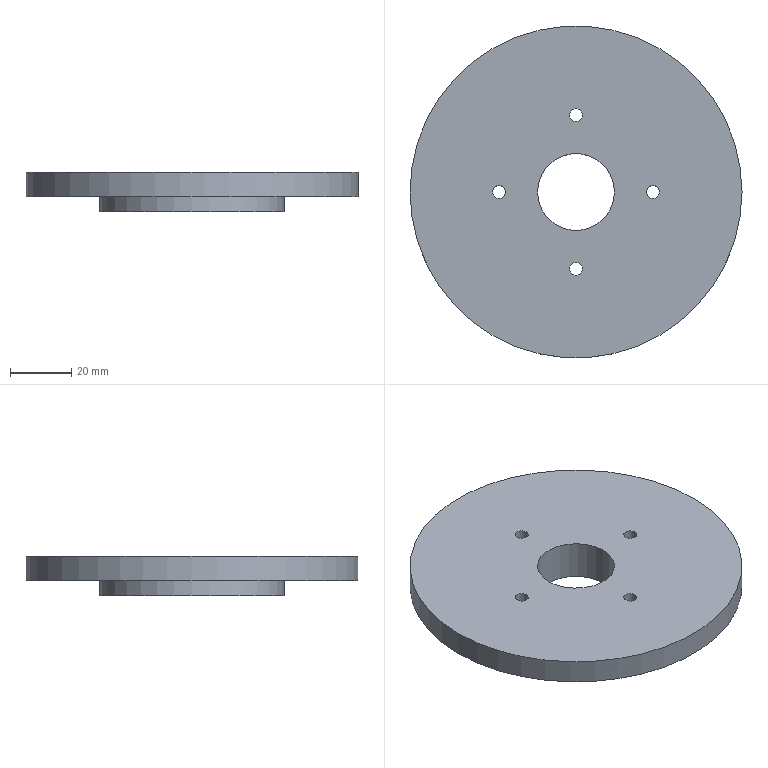NC program | NX | posted with a generic post | part box 108 x 108 x 13 mm
Whole program:
N10 G17 G21 G94 G90
(DRILLING , TOOL : ZXZ)
N12 T01 M6
N14 G54
N16 G17 G0 G90 X-25. Y0. S3000 M3
N18 G43 Z30. H1
N20 G94 G81 G98 Z-1. F200. R3.
N22 X0. Y-25.
N24 X25. Y0.
N26 X0. Y25.
N28 G80
N30 G0 X0. Y25. Z30.
N32 M5
(DRILLING_COPY , TOOL : 4.2ZT)
N34 T02 M6
N36 G54
N38 G17 G0 G90 X-25. Y0. S2000 M3
N40 G43 Z30. H2
N42 G94 G83 G98 Z-15.762 F110. Q2. R3.
N44 X0. Y-25.
N46 X25. Y0.
N48 X0. Y25.
N50 G80
N52 G0 X0. Y25. Z30.
N54 M5
(ZLEVEL_PROFILE_1_COPY_1 , TOOL : D6A45)
N56 T07 M6
N58 G54
N60 G17 G0 G90 X-25.021 Y0.012 S7500 M3
N62 G43 Z30. H7
N64 Z0.
N66 G94 G1 Z-1. F1000.
N68 X-25.924 Y0.52
N70 G3 X-26.224 Y0. R0.6
N72 X-25. Y-1.224 R1.224
N74 X-26.224 Y0. R-1.224
N76 X-25.924 Y-0.52 R0.6
N78 G1 X-25.021 Y-0.012
N80 Z0.
N82 G0 Z30.
N84 X0.012 Y25.021
N86 Z0.
N88 G1 Z-1.
N90 X0.52 Y25.924
N92 G3 X0. Y26.224 R0.6
N94 X-1.224 Y25. R1.224
N96 X0. Y26.224 R-1.224
N98 X-0.52 Y25.924 R0.6
N100 G1 X-0.012 Y25.021
N102 Z0.
N104 G0 Z30.
N106 Y-25.021
N108 Z0.
N110 G1 Z-1.
N112 X-0.52 Y-25.924
N114 G3 X0. Y-26.224 R0.6
N116 X1.224 Y-25. R1.224
N118 X0. Y-26.224 R-1.224
N120 X0.52 Y-25.924 R0.6
N122 G1 X0.012 Y-25.021
N124 Z0.
N126 G0 Z30.
N128 X25.021 Y-0.012
N130 Z0.
N132 G1 Z-1.
N134 X25.924 Y-0.52
N136 G3 X26.224 Y0. R0.6
N138 X25. Y1.224 R1.224
N140 X26.224 Y0. R-1.224
N142 X25.924 Y0.52 R0.6
N144 G1 X25.021 Y0.012
N146 Z0.
N148 G0 Z30.
N150 M5
N152 M2